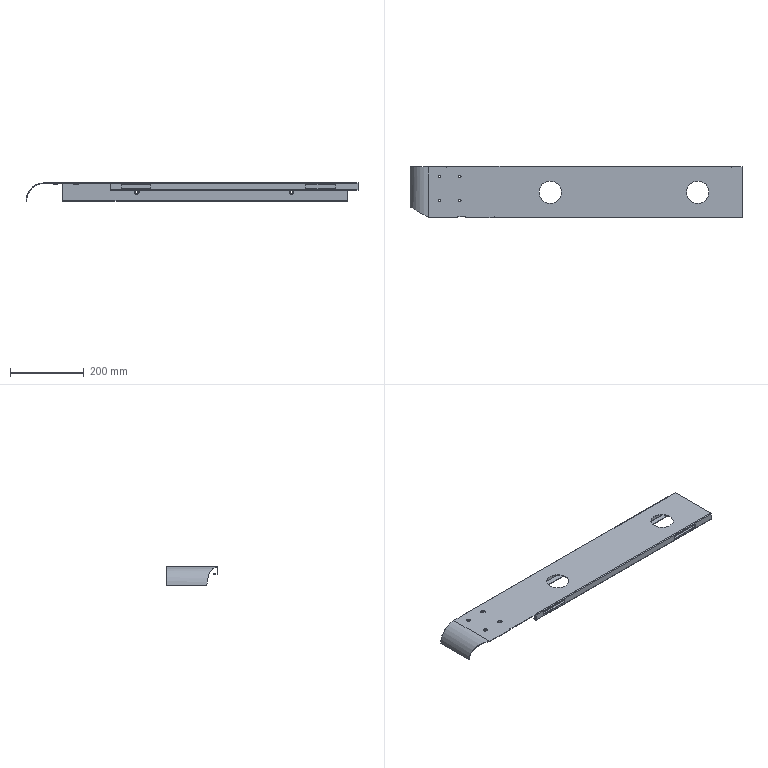Part | STEP file | FHD-021-001-E rack welded part E | 1 solid | 70 faces | box 900 x 139 x 50 mm | volume 280758 mm3 | plane 45 | cylinder 24 | spline 1 | commonest cylinder face diameters 6.8 x6 13 x6 0.4 x4 3.4 x4 60.5 x2 97 x1